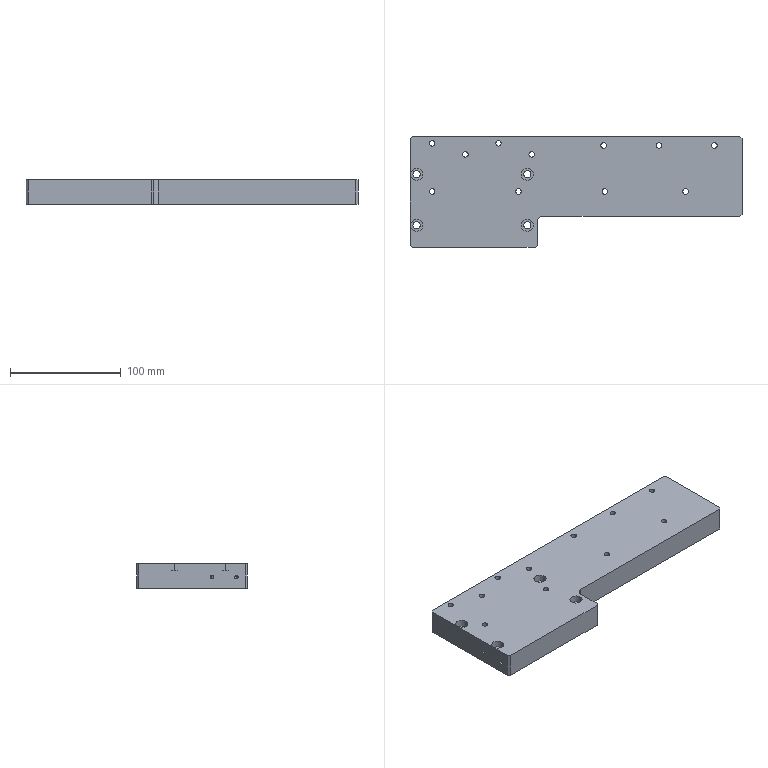Part | STEP file | 1 solid | 64 faces | box 300 x 100 x 22 mm | volume 536416 mm3 | cylinder 43 | plane 17 | cone 4 | commonest cylinder face diameters 5 x22 6.6 x8 11 x8 3.3 x4 10 x1